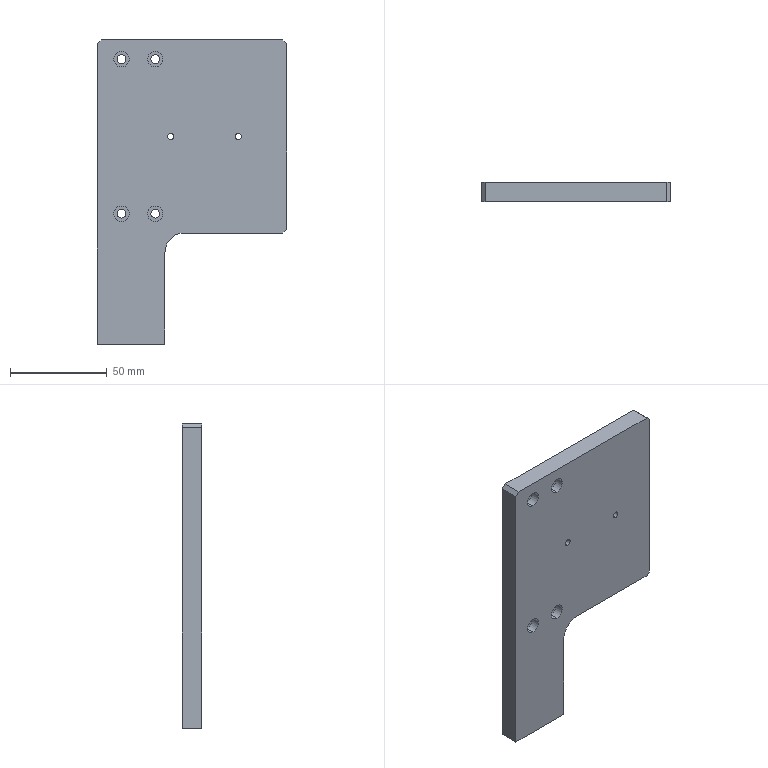Part | SolidWorks | features HoleWzd 4, Chamfer 1, Extrusion 1, Fillet 1, ICE 1 | 1 solid | 44 faces | box 98 x 10 x 157.5 mm | volume 116638 mm3 | cylinder 25 | plane 15 | cone 4 | commonest cylinder face diameters 3.3 x8 4.5 x8 8 x8 20 x1
STEP:
#1=CARTESIAN_POINT('',(23.5,0.,-97.35));
#2=VERTEX_POINT('',#1);
#3=CARTESIAN_POINT('',(23.5,0.,-100.65));
#4=VERTEX_POINT('',#3);
#5=CARTESIAN_POINT('',(23.5,0.,-99.));
#6=DIRECTION('',(1.,0.,0.));
#7=DIRECTION('',(0.,0.,-1.));
#8=AXIS2_PLACEMENT_3D('',#5,#6,#7);
#9=CIRCLE('',#8,1.65);
#10=EDGE_CURVE('',#2,#4,#9,.T.);
#11=ORIENTED_EDGE('',*,*,#10,.F.);
#12=CARTESIAN_POINT('',(35.,0.,-97.35));
#13=VERTEX_POINT('',#12);
#14=CARTESIAN_POINT('',(35.,0.,-97.35));
#15=DIRECTION('',(1.,0.,0.));
#16=VECTOR('',#15,1000.);
#17=LINE('',#14,#16);
#18=EDGE_CURVE('',#2,#13,#17,.T.);
#19=ORIENTED_EDGE('',*,*,#18,.T.);
#20=CARTESIAN_POINT('',(35.,0.,-100.65));
#21=VERTEX_POINT('',#20);
#22=CARTESIAN_POINT('',(35.,0.,-99.));
#23=DIRECTION('',(1.,0.,0.));
#24=DIRECTION('',(0.,0.,-1.));
#25=AXIS2_PLACEMENT_3D('',#22,#23,#24);
#26=CIRCLE('',#25,1.65);
#27=EDGE_CURVE('',#13,#21,#26,.T.);
#28=ORIENTED_EDGE('',*,*,#27,.T.);
#29=CARTESIAN_POINT('',(35.,0.,-100.65));
#30=DIRECTION('',(1.,0.,0.));
#31=VECTOR('',#30,1000.);
#32=LINE('',#29,#31);
#33=EDGE_CURVE('',#4,#21,#32,.T.);
#34=ORIENTED_EDGE('',*,*,#33,.F.);
#35=EDGE_LOOP('',(#11,#19,#28,#34));
#36=FACE_OUTER_BOUND('',#35,.T.);
#37=CARTESIAN_POINT('',(35.,0.,-99.));
#38=DIRECTION('',(1.,0.,0.));
#39=DIRECTION('',(0.,0.,-1.));
#40=AXIS2_PLACEMENT_3D('',#37,#38,#39);
#41=CYLINDRICAL_SURFACE('',#40,1.65);
#42=ADVANCED_FACE('',(#36),#41,.F.);
#43=CARTESIAN_POINT('',(22.509,0.,-99.));
#44=VERTEX_POINT('',#43);
#45=CARTESIAN_POINT('',(23.5,0.,-100.65));
#46=DIRECTION('',(0.515,0.,-0.8572));
#47=VECTOR('',#46,1000.);
#48=LINE('',#45,#47);
#49=EDGE_CURVE('',#44,#4,#48,.T.);
#50=ORIENTED_EDGE('',*,*,#49,.F.);
#51=CARTESIAN_POINT('',(23.5,0.,-97.35));
#52=DIRECTION('',(0.515,0.,0.8572));
#53=VECTOR('',#52,1000.);
#54=LINE('',#51,#53);
#55=EDGE_CURVE('',#44,#2,#54,.T.);
#56=ORIENTED_EDGE('',*,*,#55,.T.);
#57=ORIENTED_EDGE('',*,*,#10,.T.);
#58=EDGE_LOOP('',(#50,#56,#57));
#59=FACE_OUTER_BOUND('',#58,.T.);
#60=CARTESIAN_POINT('',(23.5,0.,-99.));
#61=DIRECTION('',(1.,0.,0.));
#62=DIRECTION('',(0.,0.,-1.));
#63=AXIS2_PLACEMENT_3D('',#60,#61,#62);
#64=CONICAL_SURFACE('',#63,1.65,1.03);
#65=ADVANCED_FACE('',(#59),#64,.F.);
#66=CARTESIAN_POINT('',(23.5,0.,-79.35));
#67=VERTEX_POINT('',#66);
#68=CARTESIAN_POINT('',(23.5,0.,-82.65));
#69=VERTEX_POINT('',#68);
#70=CARTESIAN_POINT('',(23.5,0.,-81.));
#71=DIRECTION('',(1.,0.,0.));
#72=DIRECTION('',(0.,0.,-1.));
#73=AXIS2_PLACEMENT_3D('',#70,#71,#72);
#74=CIRCLE('',#73,1.65);
#75=EDGE_CURVE('',#67,#69,#74,.T.);
#76=ORIENTED_EDGE('',*,*,#75,.F.);
#77=CARTESIAN_POINT('',(35.,0.,-79.35));
#78=VERTEX_POINT('',#77);
#79=CARTESIAN_POINT('',(35.,0.,-79.35));
#80=DIRECTION('',(1.,0.,0.));
#81=VECTOR('',#80,1000.);
#82=LINE('',#79,#81);
#83=EDGE_CURVE('',#67,#78,#82,.T.);
#84=ORIENTED_EDGE('',*,*,#83,.T.);
#85=CARTESIAN_POINT('',(35.,0.,-82.65));
#86=VERTEX_POINT('',#85);
#87=CARTESIAN_POINT('',(35.,0.,-81.));
#88=DIRECTION('',(1.,0.,0.));
#89=DIRECTION('',(0.,0.,-1.));
#90=AXIS2_PLACEMENT_3D('',#87,#88,#89);
#91=CIRCLE('',#90,1.65);
#92=EDGE_CURVE('',#78,#86,#91,.T.);
#93=ORIENTED_EDGE('',*,*,#92,.T.);
#94=CARTESIAN_POINT('',(35.,0.,-82.65));
#95=DIRECTION('',(1.,0.,0.));
#96=VECTOR('',#95,1000.);
#97=LINE('',#94,#96);
#98=EDGE_CURVE('',#69,#86,#97,.T.);
#99=ORIENTED_EDGE('',*,*,#98,.F.);
#100=EDGE_LOOP('',(#76,#84,#93,#99));
#101=FACE_OUTER_BOUND('',#100,.T.);
#102=CARTESIAN_POINT('',(35.,0.,-81.));
#103=DIRECTION('',(1.,0.,0.));
#104=DIRECTION('',(0.,0.,-1.));
#105=AXIS2_PLACEMENT_3D('',#102,#103,#104);
#106=CYLINDRICAL_SURFACE('',#105,1.65);
#107=ADVANCED_FACE('',(#101),#106,.F.);
#108=CARTESIAN_POINT('',(22.509,0.,-81.));
#109=VERTEX_POINT('',#108);
#110=CARTESIAN_POINT('',(23.5,0.,-82.65));
#111=DIRECTION('',(0.515,0.,-0.8572));
#112=VECTOR('',#111,1000.);
#113=LINE('',#110,#112);
#114=EDGE_CURVE('',#109,#69,#113,.T.);
#115=ORIENTED_EDGE('',*,*,#114,.F.);
#116=CARTESIAN_POINT('',(23.5,0.,-79.35));
#117=DIRECTION('',(0.515,0.,0.8572));
#118=VECTOR('',#117,1000.);
#119=LINE('',#116,#118);
#120=EDGE_CURVE('',#109,#67,#119,.T.);
#121=ORIENTED_EDGE('',*,*,#120,.T.);
#122=ORIENTED_EDGE('',*,*,#75,.T.);
#123=EDGE_LOOP('',(#115,#121,#122));
#124=FACE_OUTER_BOUND('',#123,.T.);
#125=CARTESIAN_POINT('',(23.5,0.,-81.));
#126=DIRECTION('',(1.,0.,0.));
#127=DIRECTION('',(0.,0.,-1.));
#128=AXIS2_PLACEMENT_3D('',#125,#126,#127);
#129=CONICAL_SURFACE('',#128,1.65,1.03);
#130=ADVANCED_FACE('',(#124),#129,.F.);
#131=CARTESIAN_POINT('',(73.,5.,1.65));
#132=VERTEX_POINT('',#131);
#133=CARTESIAN_POINT('',(73.,5.,-1.65));
#134=VERTEX_POINT('',#133);
#135=CARTESIAN_POINT('',(73.,5.,0.));
#136=DIRECTION('',(0.,-1.,0.));
#137=DIRECTION('',(0.,0.,-1.));
#138=AXIS2_PLACEMENT_3D('',#135,#136,#137);
#139=CIRCLE('',#138,1.65);
#140=EDGE_CURVE('',#132,#134,#139,.T.);
#141=ORIENTED_EDGE('',*,*,#140,.F.);
#142=CARTESIAN_POINT('',(73.,-5.,1.65));
#143=VERTEX_POINT('',#142);
#144=CARTESIAN_POINT('',(73.,-5.,1.65));
#145=DIRECTION('',(0.,-1.,0.));
#146=VECTOR('',#145,1000.);
#147=LINE('',#144,#146);
#148=EDGE_CURVE('',#132,#143,#147,.T.);
#149=ORIENTED_EDGE('',*,*,#148,.T.);
#150=CARTESIAN_POINT('',(73.,-5.,-1.65));
#151=VERTEX_POINT('',#150);
#152=CARTESIAN_POINT('',(73.,-5.,0.));
#153=DIRECTION('',(0.,-1.,0.));
#154=DIRECTION('',(0.,0.,-1.));
#155=AXIS2_PLACEMENT_3D('',#152,#153,#154);
#156=CIRCLE('',#155,1.65);
#157=EDGE_CURVE('',#143,#151,#156,.T.);
#158=ORIENTED_EDGE('',*,*,#157,.T.);
#159=CARTESIAN_POINT('',(73.,-5.,-1.65));
#160=DIRECTION('',(0.,-1.,0.));
#161=VECTOR('',#160,1000.);
#162=LINE('',#159,#161);
#163=EDGE_CURVE('',#134,#151,#162,.T.);
#164=ORIENTED_EDGE('',*,*,#163,.F.);
#165=EDGE_LOOP('',(#141,#149,#158,#164));
#166=FACE_OUTER_BOUND('',#165,.T.);
#167=CARTESIAN_POINT('',(73.,-5.,0.));
#168=DIRECTION('',(0.,-1.,0.));
#169=DIRECTION('',(0.,0.,-1.));
#170=AXIS2_PLACEMENT_3D('',#167,#168,#169);
#171=CYLINDRICAL_SURFACE('',#170,1.65);
#172=ADVANCED_FACE('',(#166),#171,.F.);
#173=CARTESIAN_POINT('',(38.,5.,1.65));
#174=VERTEX_POINT('',#173);
#175=CARTESIAN_POINT('',(38.,5.,-1.65));
#176=VERTEX_POINT('',#175);
#177=CARTESIAN_POINT('',(38.,5.,0.));
#178=DIRECTION('',(0.,-1.,0.));
#179=DIRECTION('',(0.,0.,-1.));
#180=AXIS2_PLACEMENT_3D('',#177,#178,#179);
#181=CIRCLE('',#180,1.65);
#182=EDGE_CURVE('',#174,#176,#181,.T.);
#183=ORIENTED_EDGE('',*,*,#182,.F.);
#184=CARTESIAN_POINT('',(38.,-5.,1.65));
#185=VERTEX_POINT('',#184);
#186=CARTESIAN_POINT('',(38.,-5.,1.65));
#187=DIRECTION('',(0.,-1.,0.));
#188=VECTOR('',#187,1000.);
#189=LINE('',#186,#188);
#190=EDGE_CURVE('',#174,#185,#189,.T.);
#191=ORIENTED_EDGE('',*,*,#190,.T.);
#192=CARTESIAN_POINT('',(38.,-5.,-1.65));
#193=VERTEX_POINT('',#192);
#194=CARTESIAN_POINT('',(38.,-5.,0.));
#195=DIRECTION('',(0.,-1.,0.));
#196=DIRECTION('',(0.,0.,-1.));
#197=AXIS2_PLACEMENT_3D('',#194,#195,#196);
#198=CIRCLE('',#197,1.65);
#199=EDGE_CURVE('',#185,#193,#198,.T.);
#200=ORIENTED_EDGE('',*,*,#199,.T.);
#201=CARTESIAN_POINT('',(38.,-5.,-1.65));
#202=DIRECTION('',(0.,-1.,0.));
#203=VECTOR('',#202,1000.);
#204=LINE('',#201,#203);
#205=EDGE_CURVE('',#176,#193,#204,.T.);
#206=ORIENTED_EDGE('',*,*,#205,.F.);
#207=EDGE_LOOP('',(#183,#191,#200,#206));
#208=FACE_OUTER_BOUND('',#207,.T.);
#209=CARTESIAN_POINT('',(38.,-5.,0.));
#210=DIRECTION('',(0.,-1.,0.));
#211=DIRECTION('',(0.,0.,-1.));
#212=AXIS2_PLACEMENT_3D('',#209,#210,#211);
#213=CYLINDRICAL_SURFACE('',#212,1.65);
#214=ADVANCED_FACE('',(#208),#213,.F.);
#215=CARTESIAN_POINT('',(30.,-0.4,-36.));
#216=VERTEX_POINT('',#215);
#217=CARTESIAN_POINT('',(30.,-0.4,-44.));
#218=VERTEX_POINT('',#217);
#219=CARTESIAN_POINT('',(30.,-0.4,-40.));
#220=DIRECTION('',(0.,-1.,0.));
#221=DIRECTION('',(0.,0.,-1.));
#222=AXIS2_PLACEMENT_3D('',#219,#220,#221);
#223=CIRCLE('',#222,4.);
#224=EDGE_CURVE('',#216,#218,#223,.T.);
#225=ORIENTED_EDGE('',*,*,#224,.F.);
#226=CARTESIAN_POINT('',(30.,-5.,-36.));
#227=VERTEX_POINT('',#226);
#228=CARTESIAN_POINT('',(30.,-5.,-36.));
#229=DIRECTION('',(0.,-1.,0.));
#230=VECTOR('',#229,1000.);
#231=LINE('',#228,#230);
#232=EDGE_CURVE('',#216,#227,#231,.T.);
#233=ORIENTED_EDGE('',*,*,#232,.T.);
#234=CARTESIAN_POINT('',(30.,-5.,-44.));
#235=VERTEX_POINT('',#234);
#236=CARTESIAN_POINT('',(30.,-5.,-40.));
#237=DIRECTION('',(0.,-1.,0.));
#238=DIRECTION('',(0.,0.,-1.));
#239=AXIS2_PLACEMENT_3D('',#236,#237,#238);
#240=CIRCLE('',#239,4.);
#241=EDGE_CURVE('',#227,#235,#240,.T.);
#242=ORIENTED_EDGE('',*,*,#241,.T.);
#243=CARTESIAN_POINT('',(30.,-5.,-44.));
#244=DIRECTION('',(0.,-1.,0.));
#245=VECTOR('',#244,1000.);
#246=LINE('',#243,#245);
#247=EDGE_CURVE('',#218,#235,#246,.T.);
#248=ORIENTED_EDGE('',*,*,#247,.F.);
#249=EDGE_LOOP('',(#225,#233,#242,#248));
#250=FACE_OUTER_BOUND('',#249,.T.);
#251=CARTESIAN_POINT('',(30.,-5.,-40.));
#252=DIRECTION('',(0.,-1.,0.));
#253=DIRECTION('',(0.,0.,-1.));
#254=AXIS2_PLACEMENT_3D('',#251,#252,#253);
#255=CYLINDRICAL_SURFACE('',#254,4.);
#256=ADVANCED_FACE('',(#250),#255,.F.);
#257=CARTESIAN_POINT('',(30.,5.,-37.75));
#258=VERTEX_POINT('',#257);
#259=CARTESIAN_POINT('',(30.,5.,-42.25));
#260=VERTEX_POINT('',#259);
#261=CARTESIAN_POINT('',(30.,5.,-40.));
#262=DIRECTION('',(0.,-1.,0.));
#263=DIRECTION('',(0.,0.,-1.));
#264=AXIS2_PLACEMENT_3D('',#261,#262,#263);
#265=CIRCLE('',#264,2.25);
#266=EDGE_CURVE('',#258,#260,#265,.T.);
#267=ORIENTED_EDGE('',*,*,#266,.F.);
#268=CARTESIAN_POINT('',(30.,-0.4,-37.75));
#269=VERTEX_POINT('',#268);
#270=CARTESIAN_POINT('',(30.,-5.,-37.75));
#271=DIRECTION('',(0.,-1.,0.));
#272=VECTOR('',#271,1000.);
#273=LINE('',#270,#272);
#274=EDGE_CURVE('',#258,#269,#273,.T.);
#275=ORIENTED_EDGE('',*,*,#274,.T.);
#276=CARTESIAN_POINT('',(30.,-0.4,-42.25));
#277=VERTEX_POINT('',#276);
#278=CARTESIAN_POINT('',(30.,-0.4,-40.));
#279=DIRECTION('',(0.,-1.,0.));
#280=DIRECTION('',(0.,0.,-1.));
#281=AXIS2_PLACEMENT_3D('',#278,#279,#280);
#282=CIRCLE('',#281,2.25);
#283=EDGE_CURVE('',#269,#277,#282,.T.);
#284=ORIENTED_EDGE('',*,*,#283,.T.);
#285=CARTESIAN_POINT('',(30.,-5.,-42.25));
#286=DIRECTION('',(0.,-1.,0.));
#287=VECTOR('',#286,1000.);
#288=LINE('',#285,#287);
#289=EDGE_CURVE('',#260,#277,#288,.T.);
#290=ORIENTED_EDGE('',*,*,#289,.F.);
#291=EDGE_LOOP('',(#267,#275,#284,#290));
#292=FACE_OUTER_BOUND('',#291,.T.);
#293=CARTESIAN_POINT('',(30.,-5.,-40.));
#294=DIRECTION('',(0.,-1.,0.));
#295=DIRECTION('',(0.,0.,-1.));
#296=AXIS2_PLACEMENT_3D('',#293,#294,#295);
#297=CYLINDRICAL_SURFACE('',#296,2.25);
#298=ADVANCED_FACE('',(#292),#297,.F.);
#299=CARTESIAN_POINT('',(30.,-0.4,44.));
#300=VERTEX_POINT('',#299);
#301=CARTESIAN_POINT('',(30.,-0.4,36.));
#302=VERTEX_POINT('',#301);
#303=CARTESIAN_POINT('',(30.,-0.4,40.));
#304=DIRECTION('',(0.,-1.,0.));
#305=DIRECTION('',(0.,0.,-1.));
#306=AXIS2_PLACEMENT_3D('',#303,#304,#305);
#307=CIRCLE('',#306,4.);
#308=EDGE_CURVE('',#300,#302,#307,.T.);
#309=ORIENTED_EDGE('',*,*,#308,.F.);
#310=CARTESIAN_POINT('',(30.,-5.,44.));
#311=VERTEX_POINT('',#310);
#312=CARTESIAN_POINT('',(30.,-5.,44.));
#313=DIRECTION('',(0.,-1.,0.));
#314=VECTOR('',#313,1000.);
#315=LINE('',#312,#314);
#316=EDGE_CURVE('',#300,#311,#315,.T.);
#317=ORIENTED_EDGE('',*,*,#316,.T.);
#318=CARTESIAN_POINT('',(30.,-5.,36.));
#319=VERTEX_POINT('',#318);
#320=CARTESIAN_POINT('',(30.,-5.,40.));
#321=DIRECTION('',(0.,-1.,0.));
#322=DIRECTION('',(0.,0.,-1.));
#323=AXIS2_PLACEMENT_3D('',#320,#321,#322);
#324=CIRCLE('',#323,4.);
#325=EDGE_CURVE('',#311,#319,#324,.T.);
#326=ORIENTED_EDGE('',*,*,#325,.T.);
#327=CARTESIAN_POINT('',(30.,-5.,36.));
#328=DIRECTION('',(0.,-1.,0.));
#329=VECTOR('',#328,1000.);
#330=LINE('',#327,#329);
#331=EDGE_CURVE('',#302,#319,#330,.T.);
#332=ORIENTED_EDGE('',*,*,#331,.F.);
#333=EDGE_LOOP('',(#309,#317,#326,#332));
#334=FACE_OUTER_BOUND('',#333,.T.);
#335=CARTESIAN_POINT('',(30.,-5.,40.));
#336=DIRECTION('',(0.,-1.,0.));
#337=DIRECTION('',(0.,0.,-1.));
#338=AXIS2_PLACEMENT_3D('',#335,#336,#337);
#339=CYLINDRICAL_SURFACE('',#338,4.);
#340=ADVANCED_FACE('',(#334),#339,.F.);
#341=CARTESIAN_POINT('',(30.,5.,42.25));
#342=VERTEX_POINT('',#341);
#343=CARTESIAN_POINT('',(30.,5.,37.75));
#344=VERTEX_POINT('',#343);
#345=CARTESIAN_POINT('',(30.,5.,40.));
#346=DIRECTION('',(0.,-1.,0.));
#347=DIRECTION('',(0.,0.,-1.));
#348=AXIS2_PLACEMENT_3D('',#345,#346,#347);
#349=CIRCLE('',#348,2.25);
#350=EDGE_CURVE('',#342,#344,#349,.T.);
#351=ORIENTED_EDGE('',*,*,#350,.F.);
#352=CARTESIAN_POINT('',(30.,-0.4,42.25));
#353=VERTEX_POINT('',#352);
#354=CARTESIAN_POINT('',(30.,-5.,42.25));
#355=DIRECTION('',(0.,-1.,0.));
#356=VECTOR('',#355,1000.);
#357=LINE('',#354,#356);
#358=EDGE_CURVE('',#342,#353,#357,.T.);
#359=ORIENTED_EDGE('',*,*,#358,.T.);
#360=CARTESIAN_POINT('',(30.,-0.4,37.75));
#361=VERTEX_POINT('',#360);
#362=CARTESIAN_POINT('',(30.,-0.4,40.));
#363=DIRECTION('',(0.,-1.,0.));
#364=DIRECTION('',(0.,0.,-1.));
#365=AXIS2_PLACEMENT_3D('',#362,#363,#364);
#366=CIRCLE('',#365,2.25);
#367=EDGE_CURVE('',#353,#361,#366,.T.);
#368=ORIENTED_EDGE('',*,*,#367,.T.);
#369=CARTESIAN_POINT('',(30.,-5.,37.75));
#370=DIRECTION('',(0.,-1.,0.));
#371=VECTOR('',#370,1000.);
#372=LINE('',#369,#371);
#373=EDGE_CURVE('',#344,#361,#372,.T.);
#374=ORIENTED_EDGE('',*,*,#373,.F.);
#375=EDGE_LOOP('',(#351,#359,#368,#374));
#376=FACE_OUTER_BOUND('',#375,.T.);
#377=CARTESIAN_POINT('',(30.,-5.,40.));
#378=DIRECTION('',(0.,-1.,0.));
#379=DIRECTION('',(0.,0.,-1.));
#380=AXIS2_PLACEMENT_3D('',#377,#378,#379);
#381=CYLINDRICAL_SURFACE('',#380,2.25);
#382=ADVANCED_FACE('',(#376),#381,.F.);
#383=CARTESIAN_POINT('',(12.5,-0.4,44.));
#384=VERTEX_POINT('',#383);
#385=CARTESIAN_POINT('',(12.5,-0.4,36.));
#386=VERTEX_POINT('',#385);
#387=CARTESIAN_POINT('',(12.5,-0.4,40.));
#388=DIRECTION('',(0.,-1.,0.));
#389=DIRECTION('',(0.,0.,-1.));
#390=AXIS2_PLACEMENT_3D('',#387,#388,#389);
#391=CIRCLE('',#390,4.);
#392=EDGE_CURVE('',#384,#386,#391,.T.);
#393=ORIENTED_EDGE('',*,*,#392,.F.);
#394=CARTESIAN_POINT('',(12.5,-5.,44.));
#395=VERTEX_POINT('',#394);
#396=CARTESIAN_POINT('',(12.5,-5.,44.));
#397=DIRECTION('',(0.,-1.,0.));
#398=VECTOR('',#397,1000.);
#399=LINE('',#396,#398);
#400=EDGE_CURVE('',#384,#395,#399,.T.);
#401=ORIENTED_EDGE('',*,*,#400,.T.);
#402=CARTESIAN_POINT('',(12.5,-5.,36.));
#403=VERTEX_POINT('',#402);
#404=CARTESIAN_POINT('',(12.5,-5.,40.));
#405=DIRECTION('',(0.,-1.,0.));
#406=DIRECTION('',(0.,0.,-1.));
#407=AXIS2_PLACEMENT_3D('',#404,#405,#406);
#408=CIRCLE('',#407,4.);
#409=EDGE_CURVE('',#395,#403,#408,.T.);
#410=ORIENTED_EDGE('',*,*,#409,.T.);
#411=CARTESIAN_POINT('',(12.5,-5.,36.));
#412=DIRECTION('',(0.,-1.,0.));
#413=VECTOR('',#412,1000.);
#414=LINE('',#411,#413);
#415=EDGE_CURVE('',#386,#403,#414,.T.);
#416=ORIENTED_EDGE('',*,*,#415,.F.);
#417=EDGE_LOOP('',(#393,#401,#410,#416));
#418=FACE_OUTER_BOUND('',#417,.T.);
#419=CARTESIAN_POINT('',(12.5,-5.,40.));
#420=DIRECTION('',(0.,-1.,0.));
#421=DIRECTION('',(0.,0.,-1.));
#422=AXIS2_PLACEMENT_3D('',#419,#420,#421);
#423=CYLINDRICAL_SURFACE('',#422,4.);
#424=ADVANCED_FACE('',(#418),#423,.F.);
#425=CARTESIAN_POINT('',(12.5,5.,42.25));
#426=VERTEX_POINT('',#425);
#427=CARTESIAN_POINT('',(12.5,5.,37.75));
#428=VERTEX_POINT('',#427);
#429=CARTESIAN_POINT('',(12.5,5.,40.));
#430=DIRECTION('',(0.,-1.,0.));
#431=DIRECTION('',(0.,0.,-1.));
#432=AXIS2_PLACEMENT_3D('',#429,#430,#431);
#433=CIRCLE('',#432,2.25);
#434=EDGE_CURVE('',#426,#428,#433,.T.);
#435=ORIENTED_EDGE('',*,*,#434,.F.);
#436=CARTESIAN_POINT('',(12.5,-0.4,42.25));
#437=VERTEX_POINT('',#436);
#438=CARTESIAN_POINT('',(12.5,-5.,42.25));
#439=DIRECTION('',(0.,-1.,0.));
#440=VECTOR('',#439,1000.);
#441=LINE('',#438,#440);
#442=EDGE_CURVE('',#426,#437,#441,.T.);
#443=ORIENTED_EDGE('',*,*,#442,.T.);
#444=CARTESIAN_POINT('',(12.5,-0.4,37.75));
#445=VERTEX_POINT('',#444);
#446=CARTESIAN_POINT('',(12.5,-0.4,40.));
#447=DIRECTION('',(0.,-1.,0.));
#448=DIRECTION('',(0.,0.,-1.));
#449=AXIS2_PLACEMENT_3D('',#446,#447,#448);
#450=CIRCLE('',#449,2.25);
#451=EDGE_CURVE('',#437,#445,#450,.T.);
#452=ORIENTED_EDGE('',*,*,#451,.T.);
#453=CARTESIAN_POINT('',(12.5,-5.,37.75));
#454=DIRECTION('',(0.,-1.,0.));
#455=VECTOR('',#454,1000.);
#456=LINE('',#453,#455);
#457=EDGE_CURVE('',#428,#445,#456,.T.);
#458=ORIENTED_EDGE('',*,*,#457,.F.);
#459=EDGE_LOOP('',(#435,#443,#452,#458));
#460=FACE_OUTER_BOUND('',#459,.T.);
#461=CARTESIAN_POINT('',(12.5,-5.,40.));
#462=DIRECTION('',(0.,-1.,0.));
#463=DIRECTION('',(0.,0.,-1.));
#464=AXIS2_PLACEMENT_3D('',#461,#462,#463);
#465=CYLINDRICAL_SURFACE('',#464,2.25);
#466=ADVANCED_FACE('',(#460),#465,.F.);
#467=CARTESIAN_POINT('',(12.5,-0.4,-36.));
#468=VERTEX_POINT('',#467);
#469=CARTESIAN_POINT('',(12.5,-0.4,-44.));
#470=VERTEX_POINT('',#469);
#471=CARTESIAN_POINT('',(12.5,-0.4,-40.));
#472=DIRECTION('',(0.,-1.,0.));
#473=DIRECTION('',(0.,0.,-1.));
#474=AXIS2_PLACEMENT_3D('',#471,#472,#473);
#475=CIRCLE('',#474,4.);
#476=EDGE_CURVE('',#468,#470,#475,.T.);
#477=ORIENTED_EDGE('',*,*,#476,.F.);
#478=CARTESIAN_POINT('',(12.5,-5.,-36.));
#479=VERTEX_POINT('',#478);
#480=CARTESIAN_POINT('',(12.5,-5.,-36.));
#481=DIRECTION('',(0.,-1.,0.));
#482=VECTOR('',#481,1000.);
#483=LINE('',#480,#482);
#484=EDGE_CURVE('',#468,#479,#483,.T.);
#485=ORIENTED_EDGE('',*,*,#484,.T.);
#486=CARTESIAN_POINT('',(12.5,-5.,-44.));
#487=VERTEX_POINT('',#486);
#488=CARTESIAN_POINT('',(12.5,-5.,-40.));
#489=DIRECTION('',(0.,-1.,0.));
#490=DIRECTION('',(0.,0.,-1.));
#491=AXIS2_PLACEMENT_3D('',#488,#489,#490);
#492=CIRCLE('',#491,4.);
#493=EDGE_CURVE('',#479,#487,#492,.T.);
#494=ORIENTED_EDGE('',*,*,#493,.T.);
#495=CARTESIAN_POINT('',(12.5,-5.,-44.));
#496=DIRECTION('',(0.,-1.,0.));
#497=VECTOR('',#496,1000.);
#498=LINE('',#495,#497);
#499=EDGE_CURVE('',#470,#487,#498,.T.);
#500=ORIENTED_EDGE('',*,*,#499,.F.);
#501=EDGE_LOOP('',(#477,#485,#494,#500));
#502=FACE_OUTER_BOUND('',#501,.T.);
#503=CARTESIAN_POINT('',(12.5,-5.,-40.));
#504=DIRECTION('',(0.,-1.,0.));
#505=DIRECTION('',(0.,0.,-1.));
#506=AXIS2_PLACEMENT_3D('',#503,#504,#505);
#507=CYLINDRICAL_SURFACE('',#506,4.);
#508=ADVANCED_FACE('',(#502),#507,.F.);
#509=CARTESIAN_POINT('',(12.5,5.,-37.75));
#510=VERTEX_POINT('',#509);
#511=CARTESIAN_POINT('',(12.5,5.,-42.25));
#512=VERTEX_POINT('',#511);
#513=CARTESIAN_POINT('',(12.5,5.,-40.));
#514=DIRECTION('',(0.,-1.,0.));
#515=DIRECTION('',(0.,0.,-1.));
#516=AXIS2_PLACEMENT_3D('',#513,#514,#515);
#517=CIRCLE('',#516,2.25);
#518=EDGE_CURVE('',#510,#512,#517,.T.);
#519=ORIENTED_EDGE('',*,*,#518,.F.);
#520=CARTESIAN_POINT('',(12.5,-0.4,-37.75));
#521=VERTEX_POINT('',#520);
#522=CARTESIAN_POINT('',(12.5,-5.,-37.75));
#523=DIRECTION('',(0.,-1.,0.));
#524=VECTOR('',#523,1000.);
#525=LINE('',#522,#524);
#526=EDGE_CURVE('',#510,#521,#525,.T.);
#527=ORIENTED_EDGE('',*,*,#526,.T.);
#528=CARTESIAN_POINT('',(12.5,-0.4,-42.25));
#529=VERTEX_POINT('',#528);
#530=CARTESIAN_POINT('',(12.5,-0.4,-40.));
#531=DIRECTION('',(0.,-1.,0.));
#532=DIRECTION('',(0.,0.,-1.));
#533=AXIS2_PLACEMENT_3D('',#530,#531,#532);
#534=CIRCLE('',#533,2.25);
#535=EDGE_CURVE('',#521,#529,#534,.T.);
#536=ORIENTED_EDGE('',*,*,#535,.T.);
#537=CARTESIAN_POINT('',(12.5,-5.,-42.25));
#538=DIRECTION('',(0.,-1.,0.));
#539=VECTOR('',#538,1000.);
#540=LINE('',#537,#539);
#541=EDGE_CURVE('',#512,#529,#540,.T.);
#542=ORIENTED_EDGE('',*,*,#541,.F.);
#543=EDGE_LOOP('',(#519,#527,#536,#542));
#544=FACE_OUTER_BOUND('',#543,.T.);
#545=CARTESIAN_POINT('',(12.5,-5.,-40.));
#546=DIRECTION('',(0.,-1.,0.));
#547=DIRECTION('',(0.,0.,-1.));
#548=AXIS2_PLACEMENT_3D('',#545,#546,#547);
#549=CYLINDRICAL_SURFACE('',#548,2.25);
#550=ADVANCED_FACE('',(#544),#549,.F.);
#551=CARTESIAN_POINT('',(96.,-5.,-50.));
#552=VERTEX_POINT('',#551);
#553=CARTESIAN_POINT('',(45.,-5.,-50.));
#554=VERTEX_POINT('',#553);
#555=CARTESIAN_POINT('',(98.,-5.,-50.));
#556=DIRECTION('',(-1.,0.,0.));
#557=VECTOR('',#556,1000.);
#558=LINE('',#555,#557);
#559=EDGE_CURVE('',#552,#554,#558,.T.);
#560=ORIENTED_EDGE('',*,*,#559,.T.);
#561=CARTESIAN_POINT('',(45.,5.,-50.));
#562=VERTEX_POINT('',#561);
#563=CARTESIAN_POINT('',(45.,5.,-50.));
#564=DIRECTION('',(0.,1.,0.));
#565=VECTOR('',#564,1000.);
#566=LINE('',#563,#565);
#567=EDGE_CURVE('',#554,#562,#566,.T.);
#568=ORIENTED_EDGE('',*,*,#567,.T.);
#569=CARTESIAN_POINT('',(96.,5.,-50.));
#570=VERTEX_POINT('',#569);
#571=CARTESIAN_POINT('',(98.,5.,-50.));
#572=DIRECTION('',(-1.,0.,0.));
#573=VECTOR('',#572,1000.);
#574=LINE('',#571,#573);
#575=EDGE_CURVE('',#570,#562,#574,.T.);
#576=ORIENTED_EDGE('',*,*,#575,.F.);
#577=CARTESIAN_POINT('',(96.,-5.,-50.));
#578=DIRECTION('',(0.,-1.,0.));
#579=VECTOR('',#578,1000.);
#580=LINE('',#577,#579);
#581=EDGE_CURVE('',#570,#552,#580,.T.);
#582=ORIENTED_EDGE('',*,*,#581,.T.);
#583=EDGE_LOOP('',(#560,#568,#576,#582));
#584=FACE_OUTER_BOUND('',#583,.T.);
#585=CARTESIAN_POINT('',(98.,5.,-50.));
#586=DIRECTION('',(0.,0.,1.));
#587=DIRECTION('',(1.,0.,0.));
#588=AXIS2_PLACEMENT_3D('',#585,#586,#587);
#589=PLANE('',#588);
#590=ADVANCED_FACE('',(#584),#589,.F.);
#591=ORIENTED_EDGE('',*,*,#575,.T.);
#592=CARTESIAN_POINT('',(35.,5.,-60.));
#593=VERTEX_POINT('',#592);
#594=CARTESIAN_POINT('',(45.,5.,-60.));
#595=DIRECTION('',(0.,-1.,0.));
#596=DIRECTION('',(0.,0.,-1.));
#597=AXIS2_PLACEMENT_3D('',#594,#595,#596);
#598=CIRCLE('',#597,10.);
#599=EDGE_CURVE('',#562,#593,#598,.T.);
#600=ORIENTED_EDGE('',*,*,#599,.T.);
#601=CARTESIAN_POINT('',(35.,5.,-107.5));
#602=VERTEX_POINT('',#601);
#603=CARTESIAN_POINT('',(35.,5.,-48.));
#604=DIRECTION('',(0.,0.,-1.));
#605=VECTOR('',#604,1000.);
#606=LINE('',#603,#605);
#607=EDGE_CURVE('',#593,#602,#606,.T.);
#608=ORIENTED_EDGE('',*,*,#607,.T.);
#609=CARTESIAN_POINT('',(0.,5.,-107.5));
#610=VERTEX_POINT('',#609);
#611=CARTESIAN_POINT('',(0.,5.,-107.5));
#612=DIRECTION('',(-1.,0.,0.));
#613=VECTOR('',#612,1000.);
#614=LINE('',#611,#613);
#615=EDGE_CURVE('',#602,#610,#614,.T.);
#616=ORIENTED_EDGE('',*,*,#615,.T.);
#617=CARTESIAN_POINT('',(0.,5.,48.));
#618=VERTEX_POINT('',#617);
#619=CARTESIAN_POINT('',(0.,5.,50.));
#620=DIRECTION('',(0.,0.,1.));
#621=VECTOR('',#620,1000.);
#622=LINE('',#619,#621);
#623=EDGE_CURVE('',#610,#618,#622,.T.);
#624=ORIENTED_EDGE('',*,*,#623,.T.);
#625=CARTESIAN_POINT('',(2.,5.,50.));
#626=VERTEX_POINT('',#625);
#627=CARTESIAN_POINT('',(2.,5.,50.));
#628=DIRECTION('',(0.7071,0.,0.7071));
#629=VECTOR('',#628,1000.);
#630=LINE('',#627,#629);
#631=EDGE_CURVE('',#618,#626,#630,.T.);
#632=ORIENTED_EDGE('',*,*,#631,.T.);
#633=CARTESIAN_POINT('',(96.,5.,50.));
#634=VERTEX_POINT('',#633);
#635=CARTESIAN_POINT('',(98.,5.,50.));
#636=DIRECTION('',(-1.,0.,0.));
#637=VECTOR('',#636,1000.);
#638=LINE('',#635,#637);
#639=EDGE_CURVE('',#634,#626,#638,.T.);
#640=ORIENTED_EDGE('',*,*,#639,.F.);
#641=CARTESIAN_POINT('',(98.,5.,48.));
#642=VERTEX_POINT('',#641);
#643=CARTESIAN_POINT('',(98.,5.,48.));
#644=DIRECTION('',(0.7071,0.,-0.7071));
#645=VECTOR('',#644,1000.);
#646=LINE('',#643,#645);
#647=EDGE_CURVE('',#634,#642,#646,.T.);
#648=ORIENTED_EDGE('',*,*,#647,.T.);
#649=CARTESIAN_POINT('',(98.,5.,-48.));
#650=VERTEX_POINT('',#649);
#651=CARTESIAN_POINT('',(98.,5.,50.));
#652=DIRECTION('',(0.,0.,1.));
#653=VECTOR('',#652,1000.);
#654=LINE('',#651,#653);
#655=EDGE_CURVE('',#650,#642,#654,.T.);
#656=ORIENTED_EDGE('',*,*,#655,.F.);
#657=CARTESIAN_POINT('',(98.,5.,-48.));
#658=DIRECTION('',(-0.7071,0.,-0.7071));
#659=VECTOR('',#658,1000.);
#660=LINE('',#657,#659);
#661=EDGE_CURVE('',#650,#570,#660,.T.);
#662=ORIENTED_EDGE('',*,*,#661,.T.);
#663=EDGE_LOOP('',(#591,#600,#608,#616,#624,#632,#640,#648,#656,#662));
#664=FACE_OUTER_BOUND('',#663,.T.);
#665=CARTESIAN_POINT('',(73.,5.,0.));
#666=DIRECTION('',(0.,-1.,0.));
#667=DIRECTION('',(0.,0.,-1.));
#668=AXIS2_PLACEMENT_3D('',#665,#666,#667);
#669=CIRCLE('',#668,1.65);
#670=EDGE_CURVE('',#134,#132,#669,.T.);
#671=ORIENTED_EDGE('',*,*,#670,.T.);
#672=ORIENTED_EDGE('',*,*,#140,.T.);
#673=EDGE_LOOP('',(#671,#672));
#674=FACE_BOUND('',#673,.T.);
#675=CARTESIAN_POINT('',(38.,5.,0.));
#676=DIRECTION('',(0.,-1.,0.));
#677=DIRECTION('',(0.,0.,-1.));
#678=AXIS2_PLACEMENT_3D('',#675,#676,#677);
#679=CIRCLE('',#678,1.65);
#680=EDGE_CURVE('',#176,#174,#679,.T.);
#681=ORIENTED_EDGE('',*,*,#680,.T.);
#682=ORIENTED_EDGE('',*,*,#182,.T.);
#683=EDGE_LOOP('',(#681,#682));
#684=FACE_BOUND('',#683,.T.);
#685=CARTESIAN_POINT('',(30.,5.,-40.));
#686=DIRECTION('',(0.,-1.,0.));
#687=DIRECTION('',(0.,0.,-1.));
#688=AXIS2_PLACEMENT_3D('',#685,#686,#687);
#689=CIRCLE('',#688,2.25);
#690=EDGE_CURVE('',#260,#258,#689,.T.);
#691=ORIENTED_EDGE('',*,*,#690,.T.);
#692=ORIENTED_EDGE('',*,*,#266,.T.);
#693=EDGE_LOOP('',(#691,#692));
#694=FACE_BOUND('',#693,.T.);
#695=CARTESIAN_POINT('',(30.,5.,40.));
#696=DIRECTION('',(0.,-1.,0.));
#697=DIRECTION('',(0.,0.,-1.));
#698=AXIS2_PLACEMENT_3D('',#695,#696,#697);
#699=CIRCLE('',#698,2.25);
#700=EDGE_CURVE('',#344,#342,#699,.T.);
#701=ORIENTED_EDGE('',*,*,#700,.T.);
#702=ORIENTED_EDGE('',*,*,#350,.T.);
#703=EDGE_LOOP('',(#701,#702));
#704=FACE_BOUND('',#703,.T.);
#705=CARTESIAN_POINT('',(12.5,5.,40.));
#706=DIRECTION('',(0.,-1.,0.));
#707=DIRECTION('',(0.,0.,-1.));
#708=AXIS2_PLACEMENT_3D('',#705,#706,#707);
#709=CIRCLE('',#708,2.25);
#710=EDGE_CURVE('',#428,#426,#709,.T.);
#711=ORIENTED_EDGE('',*,*,#710,.T.);
#712=ORIENTED_EDGE('',*,*,#434,.T.);
#713=EDGE_LOOP('',(#711,#712));
#714=FACE_BOUND('',#713,.T.);
#715=CARTESIAN_POINT('',(12.5,5.,-40.));
#716=DIRECTION('',(0.,-1.,0.));
#717=DIRECTION('',(0.,0.,-1.));
#718=AXIS2_PLACEMENT_3D('',#715,#716,#717);
#719=CIRCLE('',#718,2.25);
#720=EDGE_CURVE('',#512,#510,#719,.T.);
#721=ORIENTED_EDGE('',*,*,#720,.T.);
#722=ORIENTED_EDGE('',*,*,#518,.T.);
#723=EDGE_LOOP('',(#721,#722));
#724=FACE_BOUND('',#723,.T.);
#725=CARTESIAN_POINT('',(98.,5.,50.));
#726=DIRECTION('',(0.,-1.,0.));
#727=DIRECTION('',(0.,0.,-1.));
#728=AXIS2_PLACEMENT_3D('',#725,#726,#727);
#729=PLANE('',#728);
#730=ADVANCED_FACE('',(#664,#674,#684,#694,#704,#714,#724),#729,.F.);
#731=CARTESIAN_POINT('',(96.,-5.,50.));
#732=VERTEX_POINT('',#731);
#733=CARTESIAN_POINT('',(2.,-5.,50.));
#734=VERTEX_POINT('',#733);
#735=CARTESIAN_POINT('',(98.,-5.,50.));
#736=DIRECTION('',(-1.,0.,0.));
#737=VECTOR('',#736,1000.);
#738=LINE('',#735,#737);
#739=EDGE_CURVE('',#732,#734,#738,.T.);
#740=ORIENTED_EDGE('',*,*,#739,.F.);
#741=CARTESIAN_POINT('',(96.,5.,50.));
#742=DIRECTION('',(0.,1.,0.));
#743=VECTOR('',#742,1000.);
#744=LINE('',#741,#743);
#745=EDGE_CURVE('',#732,#634,#744,.T.);
#746=ORIENTED_EDGE('',*,*,#745,.T.);
#747=ORIENTED_EDGE('',*,*,#639,.T.);
#748=CARTESIAN_POINT('',(2.,5.,50.));
#749=DIRECTION('',(0.,-1.,0.));
#750=VECTOR('',#749,1000.);
#751=LINE('',#748,#750);
#752=EDGE_CURVE('',#626,#734,#751,.T.);
#753=ORIENTED_EDGE('',*,*,#752,.T.);
#754=EDGE_LOOP('',(#740,#746,#747,#753));
#755=FACE_OUTER_BOUND('',#754,.T.);
#756=CARTESIAN_POINT('',(98.,5.,50.));
#757=DIRECTION('',(0.,0.,-1.));
#758=DIRECTION('',(-1.,0.,0.));
#759=AXIS2_PLACEMENT_3D('',#756,#757,#758);
#760=PLANE('',#759);
#761=ADVANCED_FACE('',(#755),#760,.F.);
#762=CARTESIAN_POINT('',(35.,-5.,-107.5));
#763=VERTEX_POINT('',#762);
#764=CARTESIAN_POINT('',(35.,-5.,-60.));
#765=VERTEX_POINT('',#764);
#766=CARTESIAN_POINT('',(35.,-5.,-48.));
#767=DIRECTION('',(0.,0.,1.));
#768=VECTOR('',#767,1000.);
#769=LINE('',#766,#768);
#770=EDGE_CURVE('',#763,#765,#769,.T.);
#771=ORIENTED_EDGE('',*,*,#770,.T.);
#772=CARTESIAN_POINT('',(45.,-5.,-60.));
#773=DIRECTION('',(0.,1.,0.));
#774=DIRECTION('',(0.,0.,1.));
#775=AXIS2_PLACEMENT_3D('',#772,#773,#774);
#776=CIRCLE('',#775,10.);
#777=EDGE_CURVE('',#765,#554,#776,.T.);
#778=ORIENTED_EDGE('',*,*,#777,.T.);
#779=ORIENTED_EDGE('',*,*,#559,.F.);
#780=CARTESIAN_POINT('',(98.,-5.,-48.));
#781=VERTEX_POINT('',#780);
#782=CARTESIAN_POINT('',(98.,-5.,-48.));
#783=DIRECTION('',(0.7071,0.,0.7071));
#784=VECTOR('',#783,1000.);
#785=LINE('',#782,#784);
#786=EDGE_CURVE('',#552,#781,#785,.T.);
#787=ORIENTED_EDGE('',*,*,#786,.T.);
#788=CARTESIAN_POINT('',(98.,-5.,48.));
#789=VERTEX_POINT('',#788);
#790=CARTESIAN_POINT('',(98.,-5.,50.));
#791=DIRECTION('',(0.,0.,-1.));
#792=VECTOR('',#791,1000.);
#793=LINE('',#790,#792);
#794=EDGE_CURVE('',#789,#781,#793,.T.);
#795=ORIENTED_EDGE('',*,*,#794,.F.);
#796=CARTESIAN_POINT('',(98.,-5.,48.));
#797=DIRECTION('',(-0.7071,0.,0.7071));
#798=VECTOR('',#797,1000.);
#799=LINE('',#796,#798);
#800=EDGE_CURVE('',#789,#732,#799,.T.);
#801=ORIENTED_EDGE('',*,*,#800,.T.);
#802=ORIENTED_EDGE('',*,*,#739,.T.);
#803=CARTESIAN_POINT('',(0.,-5.,48.));
#804=VERTEX_POINT('',#803);
#805=CARTESIAN_POINT('',(2.,-5.,50.));
#806=DIRECTION('',(-0.7071,0.,-0.7071));
#807=VECTOR('',#806,1000.);
#808=LINE('',#805,#807);
#809=EDGE_CURVE('',#734,#804,#808,.T.);
#810=ORIENTED_EDGE('',*,*,#809,.T.);
#811=CARTESIAN_POINT('',(0.,-5.,-107.5));
#812=VERTEX_POINT('',#811);
#813=CARTESIAN_POINT('',(0.,-5.,50.));
#814=DIRECTION('',(0.,0.,-1.));
#815=VECTOR('',#814,1000.);
#816=LINE('',#813,#815);
#817=EDGE_CURVE('',#804,#812,#816,.T.);
#818=ORIENTED_EDGE('',*,*,#817,.T.);
#819=CARTESIAN_POINT('',(0.,-5.,-107.5));
#820=DIRECTION('',(1.,0.,0.));
#821=VECTOR('',#820,1000.);
#822=LINE('',#819,#821);
#823=EDGE_CURVE('',#812,#763,#822,.T.);
#824=ORIENTED_EDGE('',*,*,#823,.T.);
#825=EDGE_LOOP('',(#771,#778,#779,#787,#795,#801,#802,#810,#818,#824));
#826=FACE_OUTER_BOUND('',#825,.T.);
#827=CARTESIAN_POINT('',(73.,-5.,0.));
#828=DIRECTION('',(0.,-1.,0.));
#829=DIRECTION('',(0.,0.,-1.));
#830=AXIS2_PLACEMENT_3D('',#827,#828,#829);
#831=CIRCLE('',#830,1.65);
#832=EDGE_CURVE('',#151,#143,#831,.T.);
#833=ORIENTED_EDGE('',*,*,#832,.F.);
#834=ORIENTED_EDGE('',*,*,#157,.F.);
#835=EDGE_LOOP('',(#833,#834));
#836=FACE_BOUND('',#835,.T.);
#837=CARTESIAN_POINT('',(38.,-5.,0.));
#838=DIRECTION('',(0.,-1.,0.));
#839=DIRECTION('',(0.,0.,-1.));
#840=AXIS2_PLACEMENT_3D('',#837,#838,#839);
#841=CIRCLE('',#840,1.65);
#842=EDGE_CURVE('',#193,#185,#841,.T.);
#843=ORIENTED_EDGE('',*,*,#842,.F.);
#844=ORIENTED_EDGE('',*,*,#199,.F.);
#845=EDGE_LOOP('',(#843,#844));
#846=FACE_BOUND('',#845,.T.);
#847=CARTESIAN_POINT('',(30.,-5.,-40.));
#848=DIRECTION('',(0.,-1.,0.));
#849=DIRECTION('',(0.,0.,-1.));
#850=AXIS2_PLACEMENT_3D('',#847,#848,#849);
#851=CIRCLE('',#850,4.);
#852=EDGE_CURVE('',#235,#227,#851,.T.);
#853=ORIENTED_EDGE('',*,*,#852,.F.);
#854=ORIENTED_EDGE('',*,*,#241,.F.);
#855=EDGE_LOOP('',(#853,#854));
#856=FACE_BOUND('',#855,.T.);
#857=CARTESIAN_POINT('',(30.,-5.,40.));
#858=DIRECTION('',(0.,-1.,0.));
#859=DIRECTION('',(0.,0.,-1.));
#860=AXIS2_PLACEMENT_3D('',#857,#858,#859);
#861=CIRCLE('',#860,4.);
#862=EDGE_CURVE('',#319,#311,#861,.T.);
#863=ORIENTED_EDGE('',*,*,#862,.F.);
#864=ORIENTED_EDGE('',*,*,#325,.F.);
#865=EDGE_LOOP('',(#863,#864));
#866=FACE_BOUND('',#865,.T.);
#867=CARTESIAN_POINT('',(12.5,-5.,40.));
#868=DIRECTION('',(0.,-1.,0.));
#869=DIRECTION('',(0.,0.,-1.));
#870=AXIS2_PLACEMENT_3D('',#867,#868,#869);
#871=CIRCLE('',#870,4.);
#872=EDGE_CURVE('',#403,#395,#871,.T.);
#873=ORIENTED_EDGE('',*,*,#872,.F.);
#874=ORIENTED_EDGE('',*,*,#409,.F.);
#875=EDGE_LOOP('',(#873,#874));
#876=FACE_BOUND('',#875,.T.);
#877=CARTESIAN_POINT('',(12.5,-5.,-40.));
#878=DIRECTION('',(0.,-1.,0.));
#879=DIRECTION('',(0.,0.,-1.));
#880=AXIS2_PLACEMENT_3D('',#877,#878,#879);
#881=CIRCLE('',#880,4.);
#882=EDGE_CURVE('',#487,#479,#881,.T.);
#883=ORIENTED_EDGE('',*,*,#882,.F.);
#884=ORIENTED_EDGE('',*,*,#493,.F.);
#885=EDGE_LOOP('',(#883,#884));
#886=FACE_BOUND('',#885,.T.);
#887=CARTESIAN_POINT('',(98.,-5.,50.));
#888=DIRECTION('',(0.,1.,0.));
#889=DIRECTION('',(0.,0.,1.));
#890=AXIS2_PLACEMENT_3D('',#887,#888,#889);
#891=PLANE('',#890);
#892=ADVANCED_FACE('',(#826,#836,#846,#856,#866,#876,#886),#891,.F.);
#893=ORIENTED_EDGE('',*,*,#794,.T.);
#894=CARTESIAN_POINT('',(98.,5.,-48.));
#895=DIRECTION('',(0.,1.,0.));
#896=VECTOR('',#895,1000.);
#897=LINE('',#894,#896);
#898=EDGE_CURVE('',#781,#650,#897,.T.);
#899=ORIENTED_EDGE('',*,*,#898,.T.);
#900=ORIENTED_EDGE('',*,*,#655,.T.);
#901=CARTESIAN_POINT('',(98.,-5.,48.));
#902=DIRECTION('',(0.,-1.,0.));
#903=VECTOR('',#902,1000.);
#904=LINE('',#901,#903);
#905=EDGE_CURVE('',#642,#789,#904,.T.);
#906=ORIENTED_EDGE('',*,*,#905,.T.);
#907=EDGE_LOOP('',(#893,#899,#900,#906));
#908=FACE_OUTER_BOUND('',#907,.T.);
#909=CARTESIAN_POINT('',(98.,0.,0.));
#910=DIRECTION('',(1.,0.,0.));
#911=DIRECTION('',(0.,0.,-1.));
#912=AXIS2_PLACEMENT_3D('',#909,#910,#911);
#913=PLANE('',#912);
#914=ADVANCED_FACE('',(#908),#913,.T.);
#915=ORIENTED_EDGE('',*,*,#623,.F.);
#916=CARTESIAN_POINT('',(0.,74.031,-107.5));
#917=DIRECTION('',(0.,-1.,0.));
#918=VECTOR('',#917,1000.);
#919=LINE('',#916,#918);
#920=EDGE_CURVE('',#610,#812,#919,.T.);
#921=ORIENTED_EDGE('',*,*,#920,.T.);
#922=ORIENTED_EDGE('',*,*,#817,.F.);
#923=CARTESIAN_POINT('',(0.,0.,48.));
#924=DIRECTION('',(0.,1.,0.));
#925=VECTOR('',#924,1000.);
#926=LINE('',#923,#925);
#927=EDGE_CURVE('',#804,#618,#926,.T.);
#928=ORIENTED_EDGE('',*,*,#927,.T.);
#929=EDGE_LOOP('',(#915,#921,#922,#928));
#930=FACE_OUTER_BOUND('',#929,.T.);
#931=CARTESIAN_POINT('',(0.,0.,0.));
#932=DIRECTION('',(1.,0.,0.));
#933=DIRECTION('',(0.,0.,-1.));
#934=AXIS2_PLACEMENT_3D('',#931,#932,#933);
#935=PLANE('',#934);
#936=ADVANCED_FACE('',(#930),#935,.F.);
#937=ORIENTED_EDGE('',*,*,#526,.F.);
#938=ORIENTED_EDGE('',*,*,#720,.F.);
#939=ORIENTED_EDGE('',*,*,#541,.T.);
#940=CARTESIAN_POINT('',(12.5,-0.4,-40.));
#941=DIRECTION('',(0.,-1.,0.));
#942=DIRECTION('',(0.,0.,-1.));
#943=AXIS2_PLACEMENT_3D('',#940,#941,#942);
#944=CIRCLE('',#943,2.25);
#945=EDGE_CURVE('',#529,#521,#944,.T.);
#946=ORIENTED_EDGE('',*,*,#945,.T.);
#947=EDGE_LOOP('',(#937,#938,#939,#946));
#948=FACE_OUTER_BOUND('',#947,.T.);
#949=CARTESIAN_POINT('',(12.5,-5.,-40.));
#950=DIRECTION('',(0.,-1.,0.));
#951=DIRECTION('',(0.,0.,-1.));
#952=AXIS2_PLACEMENT_3D('',#949,#950,#951);
#953=CYLINDRICAL_SURFACE('',#952,2.25);
#954=ADVANCED_FACE('',(#948),#953,.F.);
#955=ORIENTED_EDGE('',*,*,#945,.F.);
#956=ORIENTED_EDGE('',*,*,#535,.F.);
#957=EDGE_LOOP('',(#955,#956));
#958=FACE_BOUND('',#957,.T.);
#959=CARTESIAN_POINT('',(12.5,-0.4,-40.));
#960=DIRECTION('',(0.,-1.,0.));
#961=DIRECTION('',(0.,0.,-1.));
#962=AXIS2_PLACEMENT_3D('',#959,#960,#961);
#963=CIRCLE('',#962,4.);
#964=EDGE_CURVE('',#470,#468,#963,.T.);
#965=ORIENTED_EDGE('',*,*,#964,.T.);
#966=ORIENTED_EDGE('',*,*,#476,.T.);
#967=EDGE_LOOP('',(#965,#966));
#968=FACE_OUTER_BOUND('',#967,.T.);
#969=CARTESIAN_POINT('',(14.75,-0.4,-40.));
#970=DIRECTION('',(0.,1.,0.));
#971=DIRECTION('',(0.,0.,1.));
#972=AXIS2_PLACEMENT_3D('',#969,#970,#971);
#973=PLANE('',#972);
#974=ADVANCED_FACE('',(#958,#968),#973,.F.);
#975=ORIENTED_EDGE('',*,*,#484,.F.);
#976=ORIENTED_EDGE('',*,*,#964,.F.);
#977=ORIENTED_EDGE('',*,*,#499,.T.);
#978=ORIENTED_EDGE('',*,*,#882,.T.);
#979=EDGE_LOOP('',(#975,#976,#977,#978));
#980=FACE_OUTER_BOUND('',#979,.T.);
#981=CARTESIAN_POINT('',(12.5,-5.,-40.));
#982=DIRECTION('',(0.,-1.,0.));
#983=DIRECTION('',(0.,0.,-1.));
#984=AXIS2_PLACEMENT_3D('',#981,#982,#983);
#985=CYLINDRICAL_SURFACE('',#984,4.);
#986=ADVANCED_FACE('',(#980),#985,.F.);
#987=ORIENTED_EDGE('',*,*,#442,.F.);
#988=ORIENTED_EDGE('',*,*,#710,.F.);
#989=ORIENTED_EDGE('',*,*,#457,.T.);
#990=CARTESIAN_POINT('',(12.5,-0.4,40.));
#991=DIRECTION('',(0.,-1.,0.));
#992=DIRECTION('',(0.,0.,-1.));
#993=AXIS2_PLACEMENT_3D('',#990,#991,#992);
#994=CIRCLE('',#993,2.25);
#995=EDGE_CURVE('',#445,#437,#994,.T.);
#996=ORIENTED_EDGE('',*,*,#995,.T.);
#997=EDGE_LOOP('',(#987,#988,#989,#996));
#998=FACE_OUTER_BOUND('',#997,.T.);
#999=CARTESIAN_POINT('',(12.5,-5.,40.));
#1000=DIRECTION('',(0.,-1.,0.));
#1001=DIRECTION('',(0.,0.,-1.));
#1002=AXIS2_PLACEMENT_3D('',#999,#1000,#1001);
#1003=CYLINDRICAL_SURFACE('',#1002,2.25);
#1004=ADVANCED_FACE('',(#998),#1003,.F.);
#1005=ORIENTED_EDGE('',*,*,#995,.F.);
#1006=ORIENTED_EDGE('',*,*,#451,.F.);
#1007=EDGE_LOOP('',(#1005,#1006));
#1008=FACE_BOUND('',#1007,.T.);
#1009=CARTESIAN_POINT('',(12.5,-0.4,40.));
#1010=DIRECTION('',(0.,-1.,0.));
#1011=DIRECTION('',(0.,0.,-1.));
#1012=AXIS2_PLACEMENT_3D('',#1009,#1010,#1011);
#1013=CIRCLE('',#1012,4.);
#1014=EDGE_CURVE('',#386,#384,#1013,.T.);
#1015=ORIENTED_EDGE('',*,*,#1014,.T.);
#1016=ORIENTED_EDGE('',*,*,#392,.T.);
#1017=EDGE_LOOP('',(#1015,#1016));
#1018=FACE_OUTER_BOUND('',#1017,.T.);
#1019=CARTESIAN_POINT('',(14.75,-0.4,40.));
#1020=DIRECTION('',(0.,1.,0.));
#1021=DIRECTION('',(0.,0.,1.));
#1022=AXIS2_PLACEMENT_3D('',#1019,#1020,#1021);
#1023=PLANE('',#1022);
#1024=ADVANCED_FACE('',(#1008,#1018),#1023,.F.);
#1025=ORIENTED_EDGE('',*,*,#400,.F.);
#1026=ORIENTED_EDGE('',*,*,#1014,.F.);
#1027=ORIENTED_EDGE('',*,*,#415,.T.);
#1028=ORIENTED_EDGE('',*,*,#872,.T.);
#1029=EDGE_LOOP('',(#1025,#1026,#1027,#1028));
#1030=FACE_OUTER_BOUND('',#1029,.T.);
#1031=CARTESIAN_POINT('',(12.5,-5.,40.));
#1032=DIRECTION('',(0.,-1.,0.));
#1033=DIRECTION('',(0.,0.,-1.));
#1034=AXIS2_PLACEMENT_3D('',#1031,#1032,#1033);
#1035=CYLINDRICAL_SURFACE('',#1034,4.);
#1036=ADVANCED_FACE('',(#1030),#1035,.F.);
#1037=ORIENTED_EDGE('',*,*,#358,.F.);
#1038=ORIENTED_EDGE('',*,*,#700,.F.);
#1039=ORIENTED_EDGE('',*,*,#373,.T.);
#1040=CARTESIAN_POINT('',(30.,-0.4,40.));
#1041=DIRECTION('',(0.,-1.,0.));
#1042=DIRECTION('',(0.,0.,-1.));
#1043=AXIS2_PLACEMENT_3D('',#1040,#1041,#1042);
#1044=CIRCLE('',#1043,2.25);
#1045=EDGE_CURVE('',#361,#353,#1044,.T.);
#1046=ORIENTED_EDGE('',*,*,#1045,.T.);
#1047=EDGE_LOOP('',(#1037,#1038,#1039,#1046));
#1048=FACE_OUTER_BOUND('',#1047,.T.);
#1049=CARTESIAN_POINT('',(30.,-5.,40.));
#1050=DIRECTION('',(0.,-1.,0.));
#1051=DIRECTION('',(0.,0.,-1.));
#1052=AXIS2_PLACEMENT_3D('',#1049,#1050,#1051);
#1053=CYLINDRICAL_SURFACE('',#1052,2.25);
#1054=ADVANCED_FACE('',(#1048),#1053,.F.);
#1055=ORIENTED_EDGE('',*,*,#1045,.F.);
#1056=ORIENTED_EDGE('',*,*,#367,.F.);
#1057=EDGE_LOOP('',(#1055,#1056));
#1058=FACE_BOUND('',#1057,.T.);
#1059=CARTESIAN_POINT('',(30.,-0.4,40.));
#1060=DIRECTION('',(0.,-1.,0.));
#1061=DIRECTION('',(0.,0.,-1.));
#1062=AXIS2_PLACEMENT_3D('',#1059,#1060,#1061);
#1063=CIRCLE('',#1062,4.);
#1064=EDGE_CURVE('',#302,#300,#1063,.T.);
#1065=ORIENTED_EDGE('',*,*,#1064,.T.);
#1066=ORIENTED_EDGE('',*,*,#308,.T.);
#1067=EDGE_LOOP('',(#1065,#1066));
#1068=FACE_OUTER_BOUND('',#1067,.T.);
#1069=CARTESIAN_POINT('',(32.25,-0.4,40.));
#1070=DIRECTION('',(0.,1.,0.));
#1071=DIRECTION('',(0.,0.,1.));
#1072=AXIS2_PLACEMENT_3D('',#1069,#1070,#1071);
#1073=PLANE('',#1072);
#1074=ADVANCED_FACE('',(#1058,#1068),#1073,.F.);
#1075=ORIENTED_EDGE('',*,*,#316,.F.);
#1076=ORIENTED_EDGE('',*,*,#1064,.F.);
#1077=ORIENTED_EDGE('',*,*,#331,.T.);
#1078=ORIENTED_EDGE('',*,*,#862,.T.);
#1079=EDGE_LOOP('',(#1075,#1076,#1077,#1078));
#1080=FACE_OUTER_BOUND('',#1079,.T.);
#1081=CARTESIAN_POINT('',(30.,-5.,40.));
#1082=DIRECTION('',(0.,-1.,0.));
#1083=DIRECTION('',(0.,0.,-1.));
#1084=AXIS2_PLACEMENT_3D('',#1081,#1082,#1083);
#1085=CYLINDRICAL_SURFACE('',#1084,4.);
#1086=ADVANCED_FACE('',(#1080),#1085,.F.);
#1087=ORIENTED_EDGE('',*,*,#274,.F.);
#1088=ORIENTED_EDGE('',*,*,#690,.F.);
#1089=ORIENTED_EDGE('',*,*,#289,.T.);
#1090=CARTESIAN_POINT('',(30.,-0.4,-40.));
#1091=DIRECTION('',(0.,-1.,0.));
#1092=DIRECTION('',(0.,0.,-1.));
#1093=AXIS2_PLACEMENT_3D('',#1090,#1091,#1092);
#1094=CIRCLE('',#1093,2.25);
#1095=EDGE_CURVE('',#277,#269,#1094,.T.);
#1096=ORIENTED_EDGE('',*,*,#1095,.T.);
#1097=EDGE_LOOP('',(#1087,#1088,#1089,#1096));
#1098=FACE_OUTER_BOUND('',#1097,.T.);
#1099=CARTESIAN_POINT('',(30.,-5.,-40.));
#1100=DIRECTION('',(0.,-1.,0.));
#1101=DIRECTION('',(0.,0.,-1.));
#1102=AXIS2_PLACEMENT_3D('',#1099,#1100,#1101);
#1103=CYLINDRICAL_SURFACE('',#1102,2.25);
#1104=ADVANCED_FACE('',(#1098),#1103,.F.);
#1105=ORIENTED_EDGE('',*,*,#1095,.F.);
#1106=ORIENTED_EDGE('',*,*,#283,.F.);
#1107=EDGE_LOOP('',(#1105,#1106));
#1108=FACE_BOUND('',#1107,.T.);
#1109=CARTESIAN_POINT('',(30.,-0.4,-40.));
#1110=DIRECTION('',(0.,-1.,0.));
#1111=DIRECTION('',(0.,0.,-1.));
#1112=AXIS2_PLACEMENT_3D('',#1109,#1110,#1111);
#1113=CIRCLE('',#1112,4.);
#1114=EDGE_CURVE('',#218,#216,#1113,.T.);
#1115=ORIENTED_EDGE('',*,*,#1114,.T.);
#1116=ORIENTED_EDGE('',*,*,#224,.T.);
#1117=EDGE_LOOP('',(#1115,#1116));
#1118=FACE_OUTER_BOUND('',#1117,.T.);
#1119=CARTESIAN_POINT('',(32.25,-0.4,-40.));
#1120=DIRECTION('',(0.,1.,0.));
#1121=DIRECTION('',(0.,0.,1.));
#1122=AXIS2_PLACEMENT_3D('',#1119,#1120,#1121);
#1123=PLANE('',#1122);
#1124=ADVANCED_FACE('',(#1108,#1118),#1123,.F.);
#1125=ORIENTED_EDGE('',*,*,#232,.F.);
#1126=ORIENTED_EDGE('',*,*,#1114,.F.);
#1127=ORIENTED_EDGE('',*,*,#247,.T.);
#1128=ORIENTED_EDGE('',*,*,#852,.T.);
#1129=EDGE_LOOP('',(#1125,#1126,#1127,#1128));
#1130=FACE_OUTER_BOUND('',#1129,.T.);
#1131=CARTESIAN_POINT('',(30.,-5.,-40.));
#1132=DIRECTION('',(0.,-1.,0.));
#1133=DIRECTION('',(0.,0.,-1.));
#1134=AXIS2_PLACEMENT_3D('',#1131,#1132,#1133);
#1135=CYLINDRICAL_SURFACE('',#1134,4.);
#1136=ADVANCED_FACE('',(#1130),#1135,.F.);
#1137=ORIENTED_EDGE('',*,*,#786,.F.);
#1138=ORIENTED_EDGE('',*,*,#581,.F.);
#1139=ORIENTED_EDGE('',*,*,#661,.F.);
#1140=ORIENTED_EDGE('',*,*,#898,.F.);
#1141=EDGE_LOOP('',(#1137,#1138,#1139,#1140));
#1142=FACE_OUTER_BOUND('',#1141,.T.);
#1143=CARTESIAN_POINT('',(98.,0.,-48.));
#1144=DIRECTION('',(0.7071,0.,-0.7071));
#1145=DIRECTION('',(0.,-1.,0.));
#1146=AXIS2_PLACEMENT_3D('',#1143,#1144,#1145);
#1147=PLANE('',#1146);
#1148=ADVANCED_FACE('',(#1142),#1147,.T.);
#1149=ORIENTED_EDGE('',*,*,#647,.F.);
#1150=ORIENTED_EDGE('',*,*,#745,.F.);
#1151=ORIENTED_EDGE('',*,*,#800,.F.);
#1152=ORIENTED_EDGE('',*,*,#905,.F.);
#1153=EDGE_LOOP('',(#1149,#1150,#1151,#1152));
#1154=FACE_OUTER_BOUND('',#1153,.T.);
#1155=CARTESIAN_POINT('',(98.,0.,48.));
#1156=DIRECTION('',(0.7071,0.,0.7071));
#1157=DIRECTION('',(0.,1.,0.));
#1158=AXIS2_PLACEMENT_3D('',#1155,#1156,#1157);
#1159=PLANE('',#1158);
#1160=ADVANCED_FACE('',(#1154),#1159,.T.);
#1161=ORIENTED_EDGE('',*,*,#631,.F.);
#1162=ORIENTED_EDGE('',*,*,#927,.F.);
#1163=ORIENTED_EDGE('',*,*,#809,.F.);
#1164=ORIENTED_EDGE('',*,*,#752,.F.);
#1165=EDGE_LOOP('',(#1161,#1162,#1163,#1164));
#1166=FACE_OUTER_BOUND('',#1165,.T.);
#1167=CARTESIAN_POINT('',(2.,5.,50.));
#1168=DIRECTION('',(0.7071,0.,-0.7071));
#1169=DIRECTION('',(0.,-1.,0.));
#1170=AXIS2_PLACEMENT_3D('',#1167,#1168,#1169);
#1171=PLANE('',#1170);
#1172=ADVANCED_FACE('',(#1166),#1171,.F.);
#1173=ORIENTED_EDGE('',*,*,#190,.F.);
#1174=ORIENTED_EDGE('',*,*,#680,.F.);
#1175=ORIENTED_EDGE('',*,*,#205,.T.);
#1176=ORIENTED_EDGE('',*,*,#842,.T.);
#1177=EDGE_LOOP('',(#1173,#1174,#1175,#1176));
#1178=FACE_OUTER_BOUND('',#1177,.T.);
#1179=CARTESIAN_POINT('',(38.,-5.,0.));
#1180=DIRECTION('',(0.,-1.,0.));
#1181=DIRECTION('',(0.,0.,-1.));
#1182=AXIS2_PLACEMENT_3D('',#1179,#1180,#1181);
#1183=CYLINDRICAL_SURFACE('',#1182,1.65);
#1184=ADVANCED_FACE('',(#1178),#1183,.F.);
#1185=ORIENTED_EDGE('',*,*,#148,.F.);
#1186=ORIENTED_EDGE('',*,*,#670,.F.);
#1187=ORIENTED_EDGE('',*,*,#163,.T.);
#1188=ORIENTED_EDGE('',*,*,#832,.T.);
#1189=EDGE_LOOP('',(#1185,#1186,#1187,#1188));
#1190=FACE_OUTER_BOUND('',#1189,.T.);
#1191=CARTESIAN_POINT('',(73.,-5.,0.));
#1192=DIRECTION('',(0.,-1.,0.));
#1193=DIRECTION('',(0.,0.,-1.));
#1194=AXIS2_PLACEMENT_3D('',#1191,#1192,#1193);
#1195=CYLINDRICAL_SURFACE('',#1194,1.65);
#1196=ADVANCED_FACE('',(#1190),#1195,.F.);
#1197=CARTESIAN_POINT('',(35.,0.,-99.));
#1198=DIRECTION('',(1.,0.,0.));
#1199=DIRECTION('',(0.,0.,-1.));
#1200=AXIS2_PLACEMENT_3D('',#1197,#1198,#1199);
#1201=CIRCLE('',#1200,1.65);
#1202=EDGE_CURVE('',#21,#13,#1201,.T.);
#1203=ORIENTED_EDGE('',*,*,#1202,.F.);
#1204=ORIENTED_EDGE('',*,*,#27,.F.);
#1205=EDGE_LOOP('',(#1203,#1204));
#1206=FACE_BOUND('',#1205,.T.);
#1207=CARTESIAN_POINT('',(35.,0.,-81.));
#1208=DIRECTION('',(1.,0.,0.));
#1209=DIRECTION('',(0.,0.,-1.));
#1210=AXIS2_PLACEMENT_3D('',#1207,#1208,#1209);
#1211=CIRCLE('',#1210,1.65);
#1212=EDGE_CURVE('',#86,#78,#1211,.T.);
#1213=ORIENTED_EDGE('',*,*,#1212,.F.);
#1214=ORIENTED_EDGE('',*,*,#92,.F.);
#1215=EDGE_LOOP('',(#1213,#1214));
#1216=FACE_BOUND('',#1215,.T.);
#1217=ORIENTED_EDGE('',*,*,#607,.F.);
#1218=CARTESIAN_POINT('',(35.,74.031,-60.));
#1219=DIRECTION('',(0.,-1.,0.));
#1220=VECTOR('',#1219,1000.);
#1221=LINE('',#1218,#1220);
#1222=EDGE_CURVE('',#593,#765,#1221,.T.);
#1223=ORIENTED_EDGE('',*,*,#1222,.T.);
#1224=ORIENTED_EDGE('',*,*,#770,.F.);
#1225=CARTESIAN_POINT('',(35.,74.031,-107.5));
#1226=DIRECTION('',(0.,-1.,0.));
#1227=VECTOR('',#1226,1000.);
#1228=LINE('',#1225,#1227);
#1229=EDGE_CURVE('',#602,#763,#1228,.T.);
#1230=ORIENTED_EDGE('',*,*,#1229,.F.);
#1231=EDGE_LOOP('',(#1217,#1223,#1224,#1230));
#1232=FACE_OUTER_BOUND('',#1231,.T.);
#1233=CARTESIAN_POINT('',(35.,74.031,-48.));
#1234=DIRECTION('',(1.,0.,0.));
#1235=DIRECTION('',(0.,0.,-1.));
#1236=AXIS2_PLACEMENT_3D('',#1233,#1234,#1235);
#1237=PLANE('',#1236);
#1238=ADVANCED_FACE('',(#1206,#1216,#1232),#1237,.T.);
#1239=ORIENTED_EDGE('',*,*,#615,.F.);
#1240=ORIENTED_EDGE('',*,*,#1229,.T.);
#1241=ORIENTED_EDGE('',*,*,#823,.F.);
#1242=ORIENTED_EDGE('',*,*,#920,.F.);
#1243=EDGE_LOOP('',(#1239,#1240,#1241,#1242));
#1244=FACE_OUTER_BOUND('',#1243,.T.);
#1245=CARTESIAN_POINT('',(0.,74.031,-107.5));
#1246=DIRECTION('',(0.,0.,-1.));
#1247=DIRECTION('',(-1.,0.,0.));
#1248=AXIS2_PLACEMENT_3D('',#1245,#1246,#1247);
#1249=PLANE('',#1248);
#1250=ADVANCED_FACE('',(#1244),#1249,.T.);
#1251=ORIENTED_EDGE('',*,*,#777,.F.);
#1252=ORIENTED_EDGE('',*,*,#1222,.F.);
#1253=ORIENTED_EDGE('',*,*,#599,.F.);
#1254=ORIENTED_EDGE('',*,*,#567,.F.);
#1255=EDGE_LOOP('',(#1251,#1252,#1253,#1254));
#1256=FACE_OUTER_BOUND('',#1255,.T.);
#1257=CARTESIAN_POINT('',(45.,5.,-60.));
#1258=DIRECTION('',(0.,1.,0.));
#1259=DIRECTION('',(0.,0.,1.));
#1260=AXIS2_PLACEMENT_3D('',#1257,#1258,#1259);
#1261=CYLINDRICAL_SURFACE('',#1260,10.);
#1262=ADVANCED_FACE('',(#1256),#1261,.F.);
#1263=ORIENTED_EDGE('',*,*,#120,.F.);
#1264=ORIENTED_EDGE('',*,*,#114,.T.);
#1265=CARTESIAN_POINT('',(23.5,0.,-81.));
#1266=DIRECTION('',(1.,0.,0.));
#1267=DIRECTION('',(0.,0.,-1.));
#1268=AXIS2_PLACEMENT_3D('',#1265,#1266,#1267);
#1269=CIRCLE('',#1268,1.65);
#1270=EDGE_CURVE('',#69,#67,#1269,.T.);
#1271=ORIENTED_EDGE('',*,*,#1270,.T.);
#1272=EDGE_LOOP('',(#1263,#1264,#1271));
#1273=FACE_OUTER_BOUND('',#1272,.T.);
#1274=CARTESIAN_POINT('',(23.5,0.,-81.));
#1275=DIRECTION('',(1.,0.,0.));
#1276=DIRECTION('',(0.,0.,-1.));
#1277=AXIS2_PLACEMENT_3D('',#1274,#1275,#1276);
#1278=CONICAL_SURFACE('',#1277,1.65,1.03);
#1279=ADVANCED_FACE('',(#1273),#1278,.F.);
#1280=ORIENTED_EDGE('',*,*,#83,.F.);
#1281=ORIENTED_EDGE('',*,*,#1270,.F.);
#1282=ORIENTED_EDGE('',*,*,#98,.T.);
#1283=ORIENTED_EDGE('',*,*,#1212,.T.);
#1284=EDGE_LOOP('',(#1280,#1281,#1282,#1283));
#1285=FACE_OUTER_BOUND('',#1284,.T.);
#1286=CARTESIAN_POINT('',(35.,0.,-81.));
#1287=DIRECTION('',(1.,0.,0.));
#1288=DIRECTION('',(0.,0.,-1.));
#1289=AXIS2_PLACEMENT_3D('',#1286,#1287,#1288);
#1290=CYLINDRICAL_SURFACE('',#1289,1.65);
#1291=ADVANCED_FACE('',(#1285),#1290,.F.);
#1292=ORIENTED_EDGE('',*,*,#55,.F.);
#1293=ORIENTED_EDGE('',*,*,#49,.T.);
#1294=CARTESIAN_POINT('',(23.5,0.,-99.));
#1295=DIRECTION('',(1.,0.,0.));
#1296=DIRECTION('',(0.,0.,-1.));
#1297=AXIS2_PLACEMENT_3D('',#1294,#1295,#1296);
#1298=CIRCLE('',#1297,1.65);
#1299=EDGE_CURVE('',#4,#2,#1298,.T.);
#1300=ORIENTED_EDGE('',*,*,#1299,.T.);
#1301=EDGE_LOOP('',(#1292,#1293,#1300));
#1302=FACE_OUTER_BOUND('',#1301,.T.);
#1303=CARTESIAN_POINT('',(23.5,0.,-99.));
#1304=DIRECTION('',(1.,0.,0.));
#1305=DIRECTION('',(0.,0.,-1.));
#1306=AXIS2_PLACEMENT_3D('',#1303,#1304,#1305);
#1307=CONICAL_SURFACE('',#1306,1.65,1.03);
#1308=ADVANCED_FACE('',(#1302),#1307,.F.);
#1309=ORIENTED_EDGE('',*,*,#18,.F.);
#1310=ORIENTED_EDGE('',*,*,#1299,.F.);
#1311=ORIENTED_EDGE('',*,*,#33,.T.);
#1312=ORIENTED_EDGE('',*,*,#1202,.T.);
#1313=EDGE_LOOP('',(#1309,#1310,#1311,#1312));
#1314=FACE_OUTER_BOUND('',#1313,.T.);
#1315=CARTESIAN_POINT('',(35.,0.,-99.));
#1316=DIRECTION('',(1.,0.,0.));
#1317=DIRECTION('',(0.,0.,-1.));
#1318=AXIS2_PLACEMENT_3D('',#1315,#1316,#1317);
#1319=CYLINDRICAL_SURFACE('',#1318,1.65);
#1320=ADVANCED_FACE('',(#1314),#1319,.F.);
#1321=CLOSED_SHELL('',(#42,#65,#107,#130,#172,#214,#256,#298,#340,#382,#424,#466,#508,#550,#590,#730,#761,#892,#914,#936,#954,#974,#986,#1004,#1024,#1036,#1054,#1074,#1086,#1104,#1124,#1136,#1148,#1160,#1172,#1184,#1196,#1238,#1250,#1262,#1279,#1291,#1308,#1320));
#1322=MANIFOLD_SOLID_BREP('',#1321);
#1323=CARTESIAN_POINT('',(0.,0.,0.));
#1324=DIRECTION('',(0.,0.,1.));
#1325=DIRECTION('',(1.,0.,0.));
#1326=AXIS2_PLACEMENT_3D('',#1323,#1324,#1325);
#1327=(LENGTH_UNIT()NAMED_UNIT(*)SI_UNIT(.MILLI.,.METRE.));
#1328=UNCERTAINTY_MEASURE_WITH_UNIT(LENGTH_MEASURE(0.00001),#1327,'','');
#1329=(NAMED_UNIT(*)PLANE_ANGLE_UNIT()SI_UNIT($,.RADIAN.));
#1330=(NAMED_UNIT(*)SI_UNIT($,.STERADIAN.)SOLID_ANGLE_UNIT());
#1331=(GEOMETRIC_REPRESENTATION_CONTEXT(3)GLOBAL_UNCERTAINTY_ASSIGNED_CONTEXT((#1328))GLOBAL_UNIT_ASSIGNED_CONTEXT((#1327,#1329,#1330))REPRESENTATION_CONTEXT('',''));
#1332=ADVANCED_BREP_SHAPE_REPRESENTATION('',(#1322,#1326),#1331);